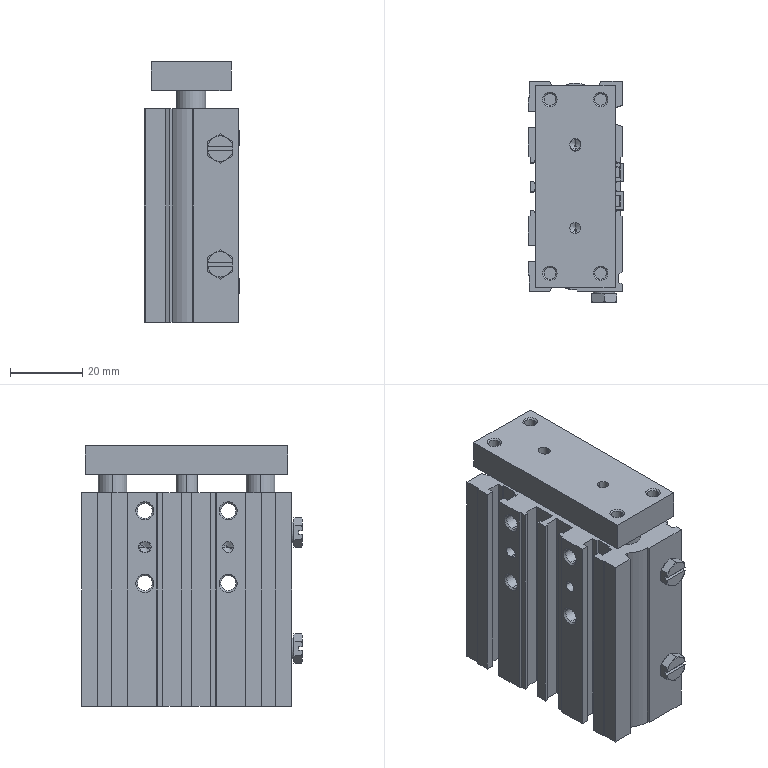Part | STEP file | MGPM12-30-M9NL_0_0_0_^Coding clamp rubber wheel | 6 solids | 463 faces | box 26.4 x 61 x 72 mm | volume 78913 mm3 | plane 235 | cylinder 128 | cone 100 | commonest cylinder face diameters 3 x18 3.242 x16 4.134 x16 8 x16 0.8 x8 2.1 x8